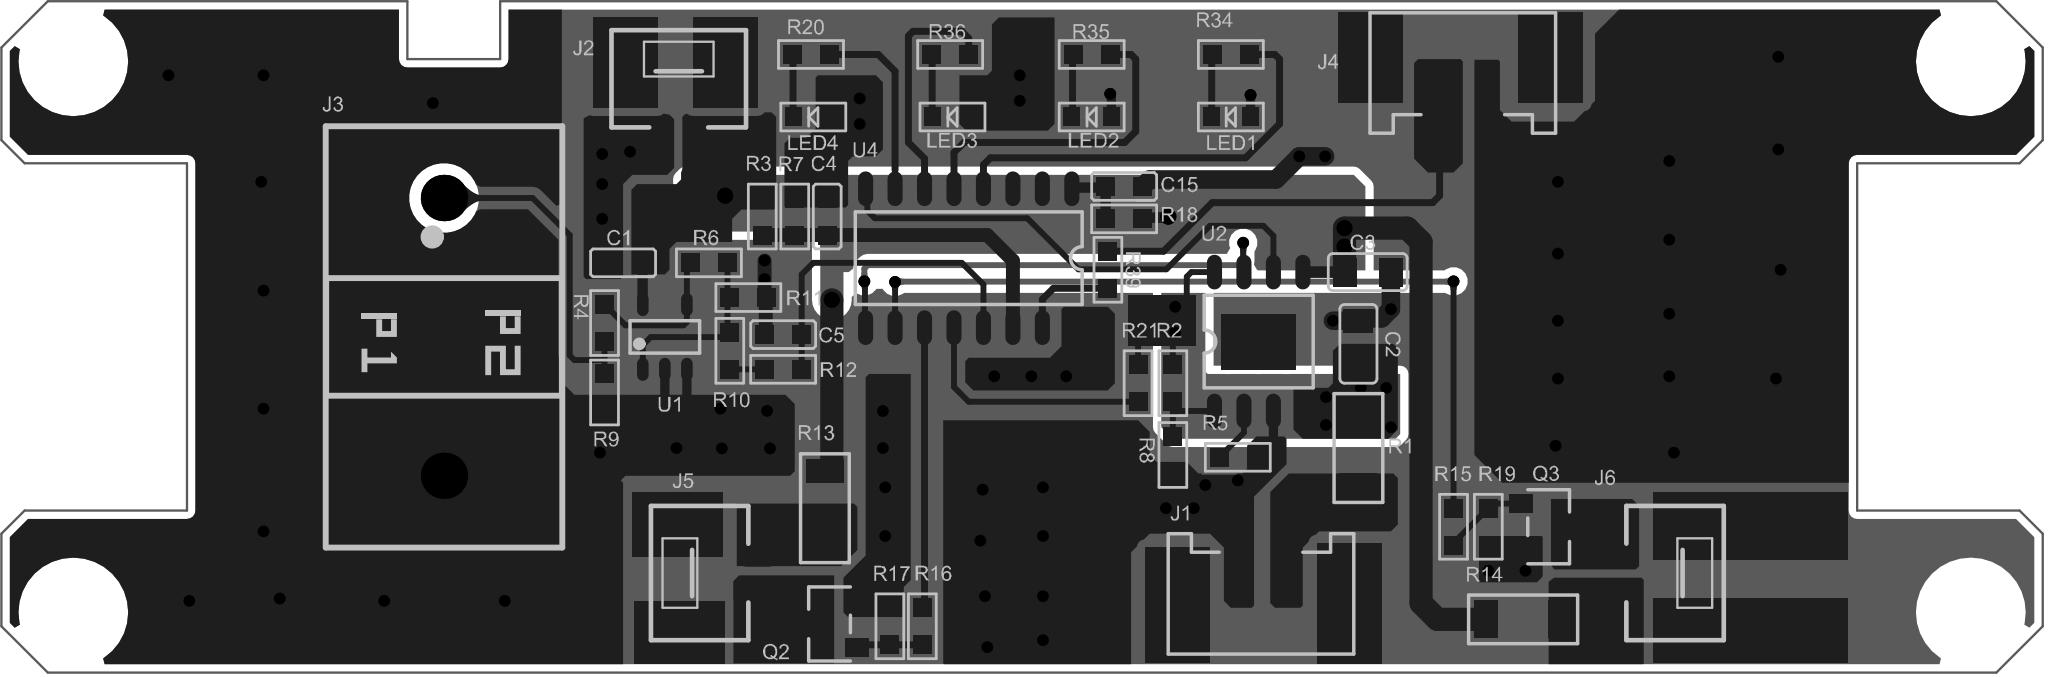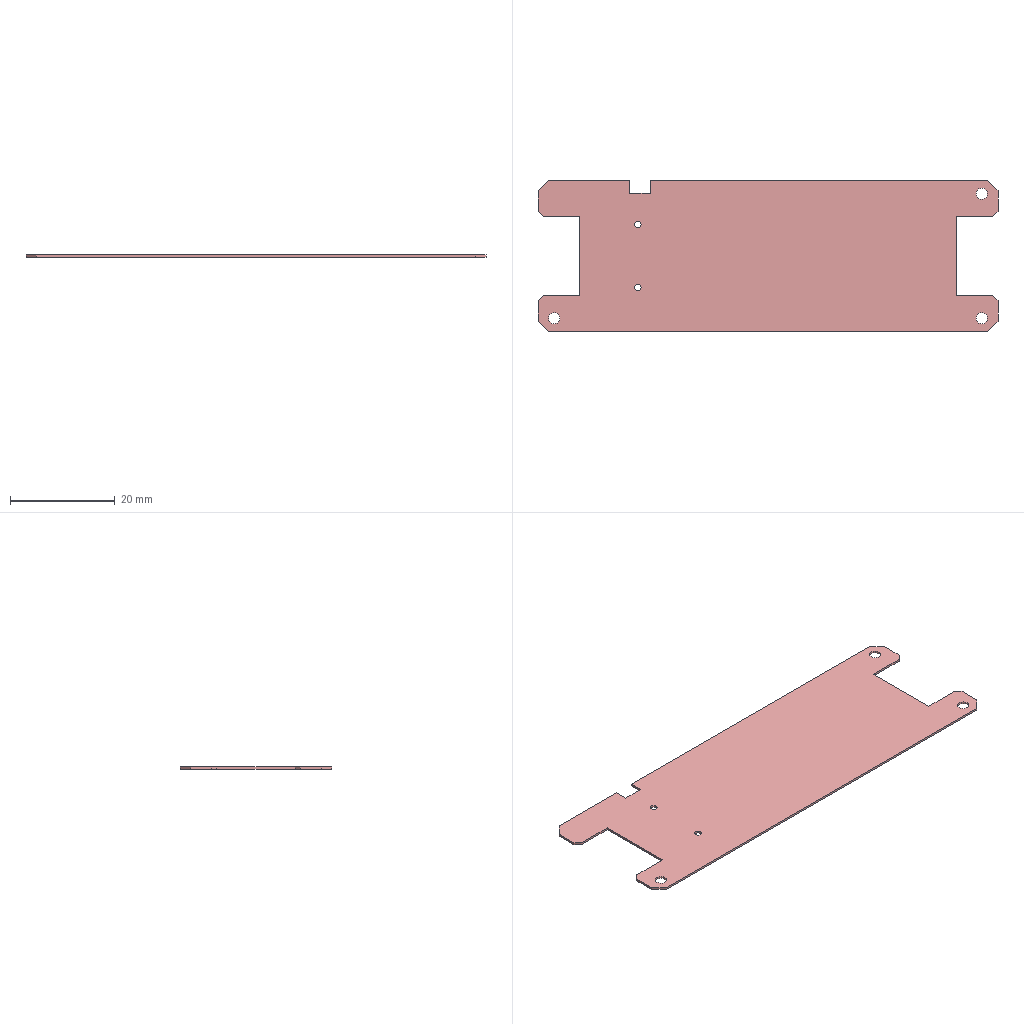Circuit board layout | Altium Designer | box 88 x 29 x 0.4 mm
Layer stack:
# Altium Designer layer stack of  (unit mm; dielectric type: 0 none, 1 core, 2 prepreg, 3 surface material)
index,name,kind,layer,copper_thickness_mm,dielectric_type,dielectric_thickness_mm,dielectric_material,dielectric_constant
0,Top Paste,other,,,,,,
1,Top Overlay,other,,,,,,
2,Top Solder,dielectric,,,3,0.0102,Solder Resist,3.5
3,Top Layer,copper,Top Layer,0.0356,,,,
4,Dielectric 1,dielectric,,,0,0.32,FR-4,4.8
5,Bottom Layer,copper,Bottom Layer,0.0356,,,,
6,Bottom Solder,dielectric,,,3,0.0102,Solder Resist,3.5
7,Bottom Overlay,other,,,,,,
8,Bottom Paste,other,,,,,,
# drill layer pairs: low layer,high layer
drill_pair,Top Layer,Bottom Layer
Part placement:
Designator,Comment,Layer,Footprint,Center-X(mm),Center-Y(mm),Rotation
C1,100nF/50V,TopLayer,C0603A,26.8,-9.3,0
U4,ZM072,TopLayer,SOP16L,41.7,-9.1,270
J3,Current sensor,TopLayer,IND-TH_L18.2-W10.2-P12.00-D0.9_ZHT103,19.08,-12.5,270
C15,1uF/10V,TopLayer,C0603A,48.4,-6,0
C3,10uF/10V,TopLayer,C0805A,58.9,-9.7,180
C2,10uF/10V,TopLayer,C0805A,58.5,-12.8,270
Q3,2N7002,TopLayer,SOT23-3L,66.7,-20.7,270
Q2,2N7002,TopLayer,SOT23-3L,35.7,-24.9,90
J6,Yellow LED,TopLayer,GH1.25-2PIN立贴带扣耐温260℃,71.125,-22.7,90
J5,Blue LED,TopLayer,GH1.25-2PIN立贴带扣耐温260℃,31.125,-22.7,270
J4,Test port,TopLayer,HY2.0WT-2A/P_Á¢Ìù´ø¿ÛÄÍÎÂ260¡æ,63,-1.9,180
J2,Battery,TopLayer,GH1.25-2PIN立贴带扣耐温260℃,29.2,-2.375,180
J1,Charge,TopLayer,HY2.0WT-2A/P_Á¢Ìù´ø¿ÛÄÍÎÂ260¡æ,54.3,-22.8,0
LED4,100%,TopLayer,LED0603A,35,-3,0
LED3,75%,TopLayer,LED0603A,41,-3,0
LED2,50%,TopLayer,LED0603A,47,-3,0
LED1,25%,TopLayer,LED0603A,53,-3,0
U2,4056,TopLayer,ESOP-8L,54.2,-12.7,90
U1,LM321,TopLayer,SOT23-5A,28.6,-12.5,90
R14,10R/1206,TopLayer,R1206A,65.6,-24.7,0
R13,10R/1206,TopLayer,R1206A,35.5,-19.9,270
R12,0R/0603,TopLayer,R0603A,33.7,-13.9,0
R11,10K/0603,TopLayer,R0603A,32.2,-10.8,0
R10,1K/0603,TopLayer,R0603A,31.4,-13.1,270
R9,2K/0603,TopLayer,R0603A,26,-14.9,270
R8,NC,TopLayer,R0603A,50.5,-17.6,90
R7,200K/0603 1%,TopLayer,R0603A,34.2,-7.3,270
R6,150K/0603,TopLayer,R0603A,30.5,-9.3,0
R5,1.2K/0603,TopLayer,R0603A,53.3,-17.7,180
R4,1K/0603,TopLayer,R0603A,26,-11.9,270
R3,510K/0603 1%,TopLayer,R0603A,32.8,-7.3,90
R2,NC,TopLayer,R0603A,50.5,-14.5,90
R1,0.5R/1206,TopLayer,R1206A,58.5,-17.3,90
C5,NC,TopLayer,C0603A,33.7,-12.4,0
C4,100nF/50V,TopLayer,C0603A,35.6,-7.3,270
R39,1K,TopLayer,R0603A,47.7,-9.6,90
R36,100R/5%,TopLayer,R0603A,40.9,-0.3,0
R35,100R/5%,TopLayer,R0603A,47,-0.3,0
R34,100R/5%,TopLayer,R0603A,53,-0.3,0
R21,NC,TopLayer,R0603A,49,-14.5,90
R20,100R/5%,TopLayer,R0603A,34.9,-0.3,0
R19,100K,TopLayer,R0603A,64.1,-20.7,90
R18,1R,TopLayer,R0603A,48.4,-7.4,180
R17,100K,TopLayer,R0603A,38.3,-25,270
R16,1K,TopLayer,R0603A,39.7,-25,90
R15,1K,TopLayer,R0603A,62.6,-20.7,90
Pad and via stacks:
# Altium Designer via and pad stacks of  (unit mm). Each distinct definition once, with the count of objects using it.
# via: kind,start_layer,end_layer,hole_mm,diameter_mm,mode(0 simple;1 top-mid-bottom;2 full stack),diameter_per_layer,count,example_net
# pad: kind,layer,hole_mm,hole_type(0 round;1 square;2 slot),plating,top_size,top_shape(1 round;2 rect;3 octagon;9 rounded rect),mid_size,bottom_size,mode,footprint,size_per_layer,count,example
pad,Top Layer,0,0,plated,0.8x0.8,2,0.8x0.8,0.8x0.8,0,R0603A,,44,R12.2
pad,Top Layer,0,0,plated,1x1.6,2,1x1.6,1x1.6,0,R1206A,,6,R14.2
pad,Top Layer,0,0,plated,1x0.5,1,1x0.5,1x0.5,0,SOT23-5A,,5,U1.1
pad,Top Layer,0,2,plated,0.65x1.5,1,0.65x1.5,0.65x1.5,0,ESOP-8L,,8,U2.7
pad,Top Layer,0,2,plated,2.4x3.2,2,2.4x3.2,2.4x3.2,0,ESOP-8L,,1,U2.0
pad,Top Layer,0,0,plated,0.7x0.8,2,0.7x0.8,0.7x0.8,0,LED0603A,,8,LED4.1
pad,Top Layer,0,0,plated,3x1.5,2,3x1.5,3x1.5,0,HY2.0WT-2A/P \u00C1\u00A2\u00CC\u00F9\u00B4\u00F8\u00BF\u00DB\u00C4\u00CD\u00CE\u00C2260\u00A1\u00E6,,4,J4.0
pad,Top Layer,0,0,plated,4.5x0.8,1,4.5x0.8,4.5x0.8,0,HY2.0WT-2A/P \u00C1\u00A2\u00CC\u00F9\u00B4\u00F8\u00BF\u00DB\u00C4\u00CD\u00CE\u00C2260\u00A1\u00E6,,4,J4.2
pad,Top Layer,0,0,plated,2.8x1.2,2,2.8x1.2,2.8x1.2,0,GH1.25-2PIN\u00C1\u00A2\u00CC\u00F9\u00B4\u00F8\u00BF\u00DB\u00C4\u00CD\u00CE\u00C2260\u00A1\u00E6,,6,J6.0
pad,Top Layer,0,0,plated,1.7x0.7,1,1.7x0.7,1.7x0.7,0,GH1.25-2PIN\u00C1\u00A2\u00CC\u00F9\u00B4\u00F8\u00BF\u00DB\u00C4\u00CD\u00CE\u00C2260\u00A1\u00E6,,6,J6.2
pad,Top Layer,0,0,plated,0.8x1,2,0.8x1,0.8x1,0,SOT23-3L,,6,Q3.3
pad,Top Layer,0,0,plated,1x1.25,2,1x1.25,1x1.25,0,C0805A,,4,C3.1
pad,Top Layer,0,2,plated,0.65x1.5,1,0.65x1.5,0.65x1.5,0,SOP16L,,16,U4.5
pad,Top Layer,0,0,plated,0.8x0.8,2,0.8x0.8,0.8x0.8,0,C0603A,,8,C1.1
pad,Top Layer,0,0,plated,1x1,1,1x1,1x1,0,,,2,3
pad,Multi-Layer,1.3,0,plated,2x2,1,2x2,2x2,0,IND-TH_L18.2-W10.2-P12.00-D0.9_ZHT103,,2,J3.2
via,Top Layer,Bottom Layer,0.3048,0.508,0,,88,GND
via,Top Layer,Bottom Layer,0.5,0.7,0,,5,BAT+
Copper pours:
name,layer,net,type(0 solid;1 hatched;2 none)
NONET_L02_P-001,Top Layer,GND,0
NONET_L02_P-001,Top Layer,GND,0
NONET_L02_P-001,Top Layer,NetJ4_2,0
NONET_L02_P-001,Top Layer,GND,0
NONET_L02_P-001,Top Layer,GND,0
NONET_L02_P-001,Top Layer,GND,0
NONET_L02_P-001,Top Layer,EN,0
NONET_L02_P-001,Top Layer,GND,0
NONET_L02_P-001,Top Layer,NetJ1_2,0
NONET_L02_P-001,Top Layer,EN,0
NONET_L02_P-001,Top Layer,NetJ6_2,0
NONET_L02_P-001,Top Layer,NetJ6_1,0
NONET_L02_P-001,Top Layer,GND,0
NONET_L02_P-001,Top Layer,GND,0
NONET_L02_P-001,Top Layer,NetJ5_1,0
NONET_L02_P-001,Top Layer,NetJ5_2,0
NONET_L02_P-001,Top Layer,BAT+,0
NONET_L02_P-001,Top Layer,GND,0
GND_L02_P015,Bottom Layer,GND,0
NONET_L02_P-001,Bottom Layer,EN,0
NONET_L02_P-001,Bottom Layer,BAT+,0
Design rules, without the lines most boards share:
# Altium Designer design rules of  (exported by Altium Designer, unit mm)
# columns: name | kind | enabled | priority | scope1 | scope2 | descriptor | typed fields (field=value)
Schematic Supply Nets | 41 | enabled | 1 | InNet('GND') | All | Supply Net(s)(InNet('GND')) |
NetAntennae | 56 | enabled | 1 | All | All | Net Antennae (Tolerance=0mm) (All) |
SilkToSilkClearance | 55 | enabled | 1 | All | All | Silk to Silk (Clearance=0mm) (All),(All) |
SilkToSolderMaskClearance | 54 | enabled | 1 | IsPad | All | Silk To Solder Mask (Clearance=0mm) (IsPad),(All) |
MinimumSolderMaskSliver | 53 | enabled | 1 | All | All | Minimum Solder Mask Sliver (Gap=0.254mm) (All),(All) |
HoleToHoleClearance | 52 | enabled | 1 | All | All | Hole To Hole Clearance (Gap=0.254mm) (All),(All) | gap=0.254
DiffPairsRouting | 51 | enabled | 1 | All | All | Differential Pairs Uncoupled Length using the Gap Constraints (Min=0.254mm) (Max=0.254mm) (Prefered=0.254mm)  and Width Constraints (Min=0.381mm) (Max=0.381mm) (Prefered=0.381mm) (All) |
HoleSize | 42 | enabled | 1 | All | All | Hole Size Constraint (Min=0.025mm) (Max=2.54mm) (All) |
Height | 50 | enabled | 1 | All | All | Height Constraint (Min=0mm) (Max=25.4mm) (Prefered=12.7mm) (All) | min_height=0 max_height=25.4
ComponentClearance | 24 | enabled | 1 | All | All | Component Clearance Constraint ( Horizontal Gap = 0.254mm, Vertical Gap = 0.254mm ) (All),(All)  | gap=0.254
SolderMaskExpansion | 13 | enabled | 1 | All | All | Solder Mask Expansion (Expansion =0.102mm) (All) | expansion=0.1016
PasteMaskExpansion | 14 | enabled | 1 | All | All | Paste Mask Expansion (Expansion =0mm) (All) | expansion=0
RoutingVias | 11 | enabled | 1 | All | All | Routing Via (MinHoleWidth=0.711mm) (MaxHoleWidth=0.711mm) (PreferredHoleWidth=0.711mm) (MinWidth=1.27mm) (MaxWidth=1.27mm) (PreferedWidth=1.27mm) (All) | via_min_hole=0.7112 via_max_hole=0.7112 via_preferred_diameter=1.27 via_preferred_hole=0.7112
RoutingCorners | 10 | enabled | 1 | All | All | Routing Corners (Style=45-Degree) (Min Setback=2.54mm) (Max Setback=2.54mm) (All) |
Width | 2 | enabled | 1 | All | All | Width Constraint (Min=0.254mm) (Max=1mm) (Preferred=0.254mm) (All) |
PolygonConnect | 20 | enabled | 1 | All | All | Polygon Connect Rule(Direct Connect )(Conductor Width=0.254mm) (Relief Angle=90 Angle) (Entries=4) (Air Gap Width=0.254mm) (All),(All) | connect_style(0=relief,1=direct,2=none)=1 relief_conductor_width=0.254 relief_entries=4
PlaneClearance | 12 | enabled | 1 | All | All | Power Plane Clearance (Clearance =0.508mm) (All) | clearance=0.508
PlaneConnect | 6 | enabled | 1 | All | All | Power Plane Connect Rule(Relief Connect )(Expansion=0.508mm) (Conductor Width=0.254mm) (Air Gap=0.254mm) (Entries=4) (All) | relief_conductor_width=0.254 relief_entries=4 relief_expansion=0.508
Clearance | 0 | enabled | 1 | All | All | Clearance Constraint (Gap=0.254mm) (All),(All) | gap=0.254
Classes set for this board:
# Altium Designer classes of  (member kind: 0 net, 1 component, 2 from-to, 3 pad, 4 layer, 5 differential pair, 6 design channel, 7 polygon, 8 structure, 9 xSignal)
# columns: class name | member kind | superclass | members
XW05 V0(YK) | 1 | no | C1; C2; C3; C4; C5; J1; J2; J3; J4; J5; J6; LED1; LED2; LED3; LED4; Q2; Q3; R1; R2; R3; R4; R5; R6; R7; R8; R9; R10; R11; R12; R13; R14; R15; R16; R17; R18; R19; R20; R21; R34; R35; R36; R39; U1; U2; U4; C4; C5; R1; R2; R3; R4; R5; R6; R7; R8; R9; R10; R11; R12; R13; R14; U1; U2; LED1; LED2; LED3; LED4; J1; J2; J4; J5; J6; Q2; Q3; C2; C3; J3; U4; C1; C15;